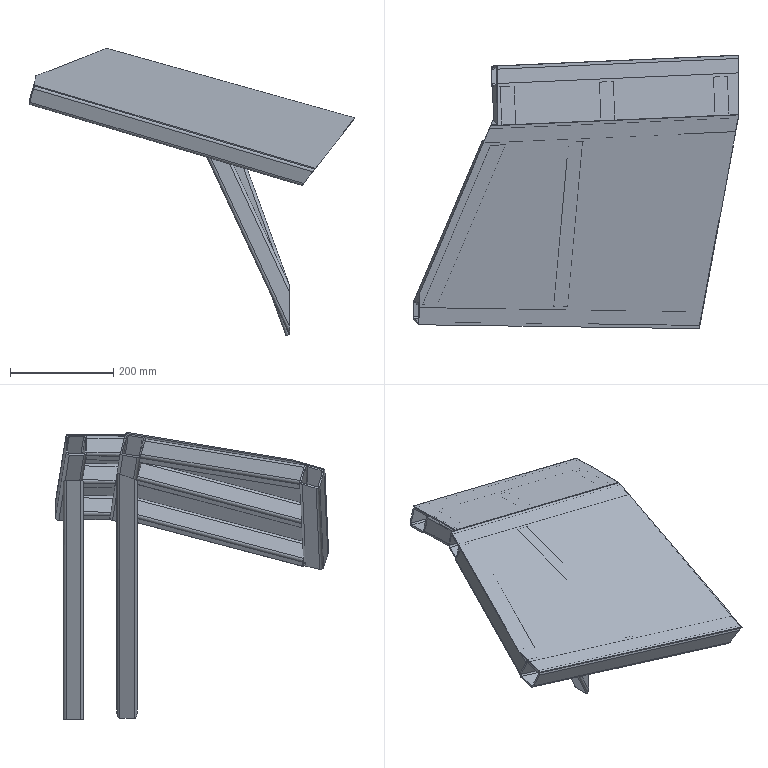Part | STEP file | _right fixed inclined baffle (down) | 13 solids | 212 faces | box 632.37 x 530.078 x 557.546 mm | volume 2099918 mm3 | plane 124 | cylinder 88 | commonest cylinder face diameters 6 x44 12 x44